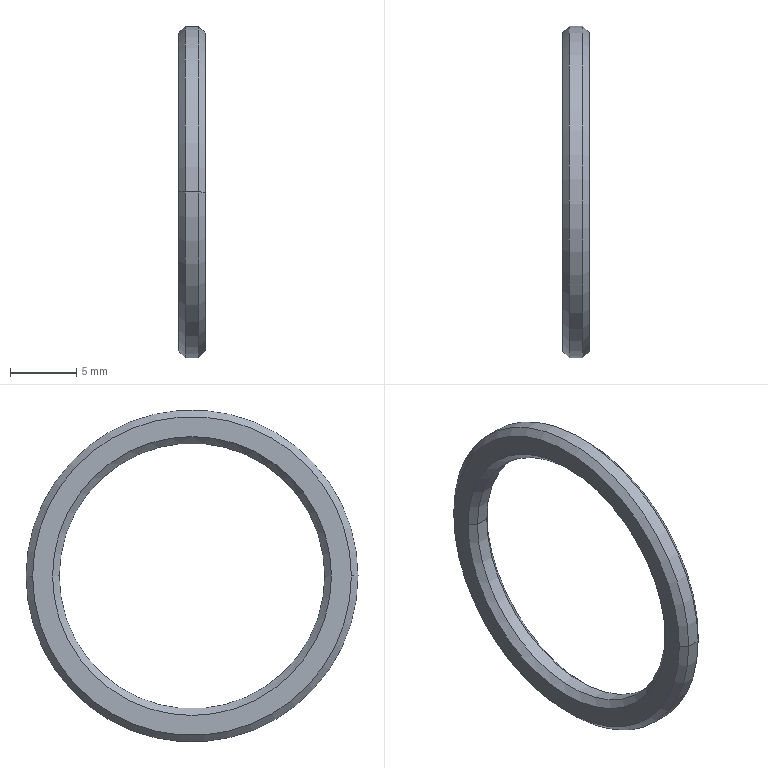Part | SolidWorks | features BaseBody 1 | 1 solid | 14 faces | box 2 x 25 x 25 mm | volume 318.086 mm3 | cone 8 | cylinder 4 | plane 2 | commonest cylinder face diameters 20 x2 25 x2
STEP:
#1=CARTESIAN_POINT('',(2.,12.,0.));
#2=VERTEX_POINT('',#1);
#3=CARTESIAN_POINT('',(2.,-12.,0.));
#4=VERTEX_POINT('',#3);
#5=CARTESIAN_POINT('',(2.,0.,0.));
#6=DIRECTION('',(1.,0.,0.));
#7=DIRECTION('',(0.,-1.,0.));
#8=AXIS2_PLACEMENT_3D('',#5,#6,#7);
#9=CIRCLE('',#8,12.);
#10=EDGE_CURVE('',#2,#4,#9,.T.);
#11=ORIENTED_EDGE('',*,*,#10,.F.);
#12=CARTESIAN_POINT('',(1.5,12.5,0.));
#13=VERTEX_POINT('',#12);
#14=CARTESIAN_POINT('',(1.5,12.5,0.));
#15=DIRECTION('',(-0.7071,0.7071,0.));
#16=VECTOR('',#15,1000.);
#17=LINE('',#14,#16);
#18=EDGE_CURVE('',#2,#13,#17,.T.);
#19=ORIENTED_EDGE('',*,*,#18,.T.);
#20=CARTESIAN_POINT('',(1.5,-12.5,0.));
#21=VERTEX_POINT('',#20);
#22=CARTESIAN_POINT('',(1.5,0.,0.));
#23=DIRECTION('',(1.,0.,0.));
#24=DIRECTION('',(0.,-1.,0.));
#25=AXIS2_PLACEMENT_3D('',#22,#23,#24);
#26=CIRCLE('',#25,12.5);
#27=EDGE_CURVE('',#13,#21,#26,.T.);
#28=ORIENTED_EDGE('',*,*,#27,.T.);
#29=CARTESIAN_POINT('',(1.5,-12.5,0.));
#30=DIRECTION('',(-0.7071,-0.7071,0.));
#31=VECTOR('',#30,1000.);
#32=LINE('',#29,#31);
#33=EDGE_CURVE('',#4,#21,#32,.T.);
#34=ORIENTED_EDGE('',*,*,#33,.F.);
#35=EDGE_LOOP('',(#11,#19,#28,#34));
#36=FACE_OUTER_BOUND('',#35,.T.);
#37=CARTESIAN_POINT('',(1.5,0.,0.));
#38=DIRECTION('',(-1.,0.,0.));
#39=DIRECTION('',(0.,-1.,0.));
#40=AXIS2_PLACEMENT_3D('',#37,#38,#39);
#41=CONICAL_SURFACE('',#40,12.5,0.7854);
#42=ADVANCED_FACE('',(#36),#41,.T.);
#43=CARTESIAN_POINT('',(1.5,-10.,0.));
#44=VERTEX_POINT('',#43);
#45=CARTESIAN_POINT('',(1.5,10.,0.));
#46=VERTEX_POINT('',#45);
#47=CARTESIAN_POINT('',(1.5,0.,0.));
#48=DIRECTION('',(1.,0.,0.));
#49=DIRECTION('',(0.,1.,0.));
#50=AXIS2_PLACEMENT_3D('',#47,#48,#49);
#51=CIRCLE('',#50,10.);
#52=EDGE_CURVE('',#44,#46,#51,.T.);
#53=ORIENTED_EDGE('',*,*,#52,.F.);
#54=CARTESIAN_POINT('',(2.,-10.5,0.));
#55=VERTEX_POINT('',#54);
#56=CARTESIAN_POINT('',(2.,-10.5,0.));
#57=DIRECTION('',(0.7071,-0.7071,0.));
#58=VECTOR('',#57,1000.);
#59=LINE('',#56,#58);
#60=EDGE_CURVE('',#44,#55,#59,.T.);
#61=ORIENTED_EDGE('',*,*,#60,.T.);
#62=CARTESIAN_POINT('',(2.,10.5,0.));
#63=VERTEX_POINT('',#62);
#64=CARTESIAN_POINT('',(2.,0.,0.));
#65=DIRECTION('',(-1.,0.,0.));
#66=DIRECTION('',(0.,1.,0.));
#67=AXIS2_PLACEMENT_3D('',#64,#65,#66);
#68=CIRCLE('',#67,10.5);
#69=EDGE_CURVE('',#63,#55,#68,.T.);
#70=ORIENTED_EDGE('',*,*,#69,.F.);
#71=CARTESIAN_POINT('',(2.,10.5,0.));
#72=DIRECTION('',(0.7071,0.7071,0.));
#73=VECTOR('',#72,1000.);
#74=LINE('',#71,#73);
#75=EDGE_CURVE('',#46,#63,#74,.T.);
#76=ORIENTED_EDGE('',*,*,#75,.F.);
#77=EDGE_LOOP('',(#53,#61,#70,#76));
#78=FACE_OUTER_BOUND('',#77,.T.);
#79=CARTESIAN_POINT('',(2.,0.,0.));
#80=DIRECTION('',(1.,0.,0.));
#81=DIRECTION('',(0.,1.,0.));
#82=AXIS2_PLACEMENT_3D('',#79,#80,#81);
#83=CONICAL_SURFACE('',#82,10.5,0.7854);
#84=ADVANCED_FACE('',(#78),#83,.F.);
#85=CARTESIAN_POINT('',(0.5,12.5,0.));
#86=VERTEX_POINT('',#85);
#87=CARTESIAN_POINT('',(0.5,-12.5,0.));
#88=VERTEX_POINT('',#87);
#89=CARTESIAN_POINT('',(0.5,0.,0.));
#90=DIRECTION('',(1.,0.,0.));
#91=DIRECTION('',(0.,1.,0.));
#92=AXIS2_PLACEMENT_3D('',#89,#90,#91);
#93=CIRCLE('',#92,12.5);
#94=EDGE_CURVE('',#86,#88,#93,.T.);
#95=ORIENTED_EDGE('',*,*,#94,.T.);
#96=CARTESIAN_POINT('',(-3.,-12.5,0.));
#97=DIRECTION('',(1.,0.,0.));
#98=VECTOR('',#97,1000.);
#99=LINE('',#96,#98);
#100=EDGE_CURVE('',#88,#21,#99,.T.);
#101=ORIENTED_EDGE('',*,*,#100,.T.);
#102=ORIENTED_EDGE('',*,*,#27,.F.);
#103=CARTESIAN_POINT('',(-3.,12.5,0.));
#104=DIRECTION('',(1.,0.,0.));
#105=VECTOR('',#104,1000.);
#106=LINE('',#103,#105);
#107=EDGE_CURVE('',#86,#13,#106,.T.);
#108=ORIENTED_EDGE('',*,*,#107,.F.);
#109=EDGE_LOOP('',(#95,#101,#102,#108));
#110=FACE_OUTER_BOUND('',#109,.T.);
#111=CARTESIAN_POINT('',(-3.,0.,0.));
#112=DIRECTION('',(1.,0.,0.));
#113=DIRECTION('',(0.,1.,0.));
#114=AXIS2_PLACEMENT_3D('',#111,#112,#113);
#115=CYLINDRICAL_SURFACE('',#114,12.5);
#116=ADVANCED_FACE('',(#110),#115,.T.);
#117=CARTESIAN_POINT('',(0.5,-10.,0.));
#118=VERTEX_POINT('',#117);
#119=CARTESIAN_POINT('',(0.5,10.,0.));
#120=VERTEX_POINT('',#119);
#121=CARTESIAN_POINT('',(0.5,0.,0.));
#122=DIRECTION('',(1.,0.,0.));
#123=DIRECTION('',(0.,1.,0.));
#124=AXIS2_PLACEMENT_3D('',#121,#122,#123);
#125=CIRCLE('',#124,10.);
#126=EDGE_CURVE('',#118,#120,#125,.T.);
#127=ORIENTED_EDGE('',*,*,#126,.F.);
#128=CARTESIAN_POINT('',(-3.,-10.,0.));
#129=DIRECTION('',(1.,0.,0.));
#130=VECTOR('',#129,1000.);
#131=LINE('',#128,#130);
#132=EDGE_CURVE('',#118,#44,#131,.T.);
#133=ORIENTED_EDGE('',*,*,#132,.T.);
#134=ORIENTED_EDGE('',*,*,#52,.T.);
#135=CARTESIAN_POINT('',(-3.,10.,0.));
#136=DIRECTION('',(1.,0.,0.));
#137=VECTOR('',#136,1000.);
#138=LINE('',#135,#137);
#139=EDGE_CURVE('',#120,#46,#138,.T.);
#140=ORIENTED_EDGE('',*,*,#139,.F.);
#141=EDGE_LOOP('',(#127,#133,#134,#140));
#142=FACE_OUTER_BOUND('',#141,.T.);
#143=CARTESIAN_POINT('',(-3.,0.,0.));
#144=DIRECTION('',(1.,0.,0.));
#145=DIRECTION('',(0.,1.,0.));
#146=AXIS2_PLACEMENT_3D('',#143,#144,#145);
#147=CYLINDRICAL_SURFACE('',#146,10.);
#148=ADVANCED_FACE('',(#142),#147,.F.);
#149=CARTESIAN_POINT('',(0.,12.,0.));
#150=VERTEX_POINT('',#149);
#151=CARTESIAN_POINT('',(0.,-12.,0.));
#152=VERTEX_POINT('',#151);
#153=CARTESIAN_POINT('',(0.,0.,0.));
#154=DIRECTION('',(1.,0.,0.));
#155=DIRECTION('',(0.,1.,0.));
#156=AXIS2_PLACEMENT_3D('',#153,#154,#155);
#157=CIRCLE('',#156,12.);
#158=EDGE_CURVE('',#150,#152,#157,.T.);
#159=ORIENTED_EDGE('',*,*,#158,.T.);
#160=CARTESIAN_POINT('',(0.5,-12.5,0.));
#161=DIRECTION('',(0.7071,-0.7071,0.));
#162=VECTOR('',#161,1000.);
#163=LINE('',#160,#162);
#164=EDGE_CURVE('',#152,#88,#163,.T.);
#165=ORIENTED_EDGE('',*,*,#164,.T.);
#166=ORIENTED_EDGE('',*,*,#94,.F.);
#167=CARTESIAN_POINT('',(0.5,12.5,0.));
#168=DIRECTION('',(0.7071,0.7071,0.));
#169=VECTOR('',#168,1000.);
#170=LINE('',#167,#169);
#171=EDGE_CURVE('',#150,#86,#170,.T.);
#172=ORIENTED_EDGE('',*,*,#171,.F.);
#173=EDGE_LOOP('',(#159,#165,#166,#172));
#174=FACE_OUTER_BOUND('',#173,.T.);
#175=CARTESIAN_POINT('',(0.5,0.,0.));
#176=DIRECTION('',(1.,0.,0.));
#177=DIRECTION('',(0.,1.,0.));
#178=AXIS2_PLACEMENT_3D('',#175,#176,#177);
#179=CONICAL_SURFACE('',#178,12.5,0.7854);
#180=ADVANCED_FACE('',(#174),#179,.T.);
#181=ORIENTED_EDGE('',*,*,#126,.T.);
#182=CARTESIAN_POINT('',(0.,10.5,0.));
#183=VERTEX_POINT('',#182);
#184=CARTESIAN_POINT('',(0.,10.5,0.));
#185=DIRECTION('',(-0.7071,0.7071,0.));
#186=VECTOR('',#185,1000.);
#187=LINE('',#184,#186);
#188=EDGE_CURVE('',#120,#183,#187,.T.);
#189=ORIENTED_EDGE('',*,*,#188,.T.);
#190=CARTESIAN_POINT('',(0.,-10.5,0.));
#191=VERTEX_POINT('',#190);
#192=CARTESIAN_POINT('',(0.,0.,0.));
#193=DIRECTION('',(1.,0.,0.));
#194=DIRECTION('',(0.,-1.,0.));
#195=AXIS2_PLACEMENT_3D('',#192,#193,#194);
#196=CIRCLE('',#195,10.5);
#197=EDGE_CURVE('',#191,#183,#196,.T.);
#198=ORIENTED_EDGE('',*,*,#197,.F.);
#199=CARTESIAN_POINT('',(0.,-10.5,0.));
#200=DIRECTION('',(-0.7071,-0.7071,0.));
#201=VECTOR('',#200,1000.);
#202=LINE('',#199,#201);
#203=EDGE_CURVE('',#118,#191,#202,.T.);
#204=ORIENTED_EDGE('',*,*,#203,.F.);
#205=EDGE_LOOP('',(#181,#189,#198,#204));
#206=FACE_OUTER_BOUND('',#205,.T.);
#207=CARTESIAN_POINT('',(0.,0.,0.));
#208=DIRECTION('',(-1.,0.,0.));
#209=DIRECTION('',(0.,-1.,0.));
#210=AXIS2_PLACEMENT_3D('',#207,#208,#209);
#211=CONICAL_SURFACE('',#210,10.5,0.7854);
#212=ADVANCED_FACE('',(#206),#211,.F.);
#213=ORIENTED_EDGE('',*,*,#197,.T.);
#214=CARTESIAN_POINT('',(0.,0.,0.));
#215=DIRECTION('',(1.,0.,0.));
#216=DIRECTION('',(0.,-1.,0.));
#217=AXIS2_PLACEMENT_3D('',#214,#215,#216);
#218=CIRCLE('',#217,10.5);
#219=EDGE_CURVE('',#183,#191,#218,.T.);
#220=ORIENTED_EDGE('',*,*,#219,.T.);
#221=EDGE_LOOP('',(#213,#220));
#222=FACE_BOUND('',#221,.T.);
#223=ORIENTED_EDGE('',*,*,#158,.F.);
#224=CARTESIAN_POINT('',(0.,0.,0.));
#225=DIRECTION('',(1.,0.,0.));
#226=DIRECTION('',(0.,1.,0.));
#227=AXIS2_PLACEMENT_3D('',#224,#225,#226);
#228=CIRCLE('',#227,12.);
#229=EDGE_CURVE('',#152,#150,#228,.T.);
#230=ORIENTED_EDGE('',*,*,#229,.F.);
#231=EDGE_LOOP('',(#223,#230));
#232=FACE_OUTER_BOUND('',#231,.T.);
#233=CARTESIAN_POINT('',(0.,-10.5,0.));
#234=DIRECTION('',(-1.,0.,0.));
#235=DIRECTION('',(0.,1.,0.));
#236=AXIS2_PLACEMENT_3D('',#233,#234,#235);
#237=PLANE('',#236);
#238=ADVANCED_FACE('',(#222,#232),#237,.T.);
#239=ORIENTED_EDGE('',*,*,#69,.T.);
#240=CARTESIAN_POINT('',(2.,0.,0.));
#241=DIRECTION('',(-1.,0.,0.));
#242=DIRECTION('',(0.,1.,0.));
#243=AXIS2_PLACEMENT_3D('',#240,#241,#242);
#244=CIRCLE('',#243,10.5);
#245=EDGE_CURVE('',#55,#63,#244,.T.);
#246=ORIENTED_EDGE('',*,*,#245,.T.);
#247=EDGE_LOOP('',(#239,#246));
#248=FACE_BOUND('',#247,.T.);
#249=CARTESIAN_POINT('',(2.,0.,0.));
#250=DIRECTION('',(1.,0.,0.));
#251=DIRECTION('',(0.,-1.,0.));
#252=AXIS2_PLACEMENT_3D('',#249,#250,#251);
#253=CIRCLE('',#252,12.);
#254=EDGE_CURVE('',#4,#2,#253,.T.);
#255=ORIENTED_EDGE('',*,*,#254,.T.);
#256=ORIENTED_EDGE('',*,*,#10,.T.);
#257=EDGE_LOOP('',(#255,#256));
#258=FACE_OUTER_BOUND('',#257,.T.);
#259=CARTESIAN_POINT('',(2.,-12.,0.));
#260=DIRECTION('',(1.,0.,0.));
#261=DIRECTION('',(0.,1.,0.));
#262=AXIS2_PLACEMENT_3D('',#259,#260,#261);
#263=PLANE('',#262);
#264=ADVANCED_FACE('',(#248,#258),#263,.T.);
#265=ORIENTED_EDGE('',*,*,#188,.F.);
#266=CARTESIAN_POINT('',(0.5,0.,0.));
#267=DIRECTION('',(1.,0.,0.));
#268=DIRECTION('',(0.,1.,0.));
#269=AXIS2_PLACEMENT_3D('',#266,#267,#268);
#270=CIRCLE('',#269,10.);
#271=EDGE_CURVE('',#120,#118,#270,.T.);
#272=ORIENTED_EDGE('',*,*,#271,.T.);
#273=ORIENTED_EDGE('',*,*,#203,.T.);
#274=ORIENTED_EDGE('',*,*,#219,.F.);
#275=EDGE_LOOP('',(#265,#272,#273,#274));
#276=FACE_OUTER_BOUND('',#275,.T.);
#277=CARTESIAN_POINT('',(0.,0.,0.));
#278=DIRECTION('',(-1.,0.,0.));
#279=DIRECTION('',(0.,-1.,0.));
#280=AXIS2_PLACEMENT_3D('',#277,#278,#279);
#281=CONICAL_SURFACE('',#280,10.5,0.7854);
#282=ADVANCED_FACE('',(#276),#281,.F.);
#283=ORIENTED_EDGE('',*,*,#164,.F.);
#284=ORIENTED_EDGE('',*,*,#229,.T.);
#285=ORIENTED_EDGE('',*,*,#171,.T.);
#286=CARTESIAN_POINT('',(0.5,0.,0.));
#287=DIRECTION('',(1.,0.,0.));
#288=DIRECTION('',(0.,1.,0.));
#289=AXIS2_PLACEMENT_3D('',#286,#287,#288);
#290=CIRCLE('',#289,12.5);
#291=EDGE_CURVE('',#88,#86,#290,.T.);
#292=ORIENTED_EDGE('',*,*,#291,.F.);
#293=EDGE_LOOP('',(#283,#284,#285,#292));
#294=FACE_OUTER_BOUND('',#293,.T.);
#295=CARTESIAN_POINT('',(0.5,0.,0.));
#296=DIRECTION('',(1.,0.,0.));
#297=DIRECTION('',(0.,1.,0.));
#298=AXIS2_PLACEMENT_3D('',#295,#296,#297);
#299=CONICAL_SURFACE('',#298,12.5,0.7854);
#300=ADVANCED_FACE('',(#294),#299,.T.);
#301=ORIENTED_EDGE('',*,*,#132,.F.);
#302=ORIENTED_EDGE('',*,*,#271,.F.);
#303=ORIENTED_EDGE('',*,*,#139,.T.);
#304=CARTESIAN_POINT('',(1.5,0.,0.));
#305=DIRECTION('',(1.,0.,0.));
#306=DIRECTION('',(0.,1.,0.));
#307=AXIS2_PLACEMENT_3D('',#304,#305,#306);
#308=CIRCLE('',#307,10.);
#309=EDGE_CURVE('',#46,#44,#308,.T.);
#310=ORIENTED_EDGE('',*,*,#309,.T.);
#311=EDGE_LOOP('',(#301,#302,#303,#310));
#312=FACE_OUTER_BOUND('',#311,.T.);
#313=CARTESIAN_POINT('',(-3.,0.,0.));
#314=DIRECTION('',(1.,0.,0.));
#315=DIRECTION('',(0.,1.,0.));
#316=AXIS2_PLACEMENT_3D('',#313,#314,#315);
#317=CYLINDRICAL_SURFACE('',#316,10.);
#318=ADVANCED_FACE('',(#312),#317,.F.);
#319=ORIENTED_EDGE('',*,*,#100,.F.);
#320=ORIENTED_EDGE('',*,*,#291,.T.);
#321=ORIENTED_EDGE('',*,*,#107,.T.);
#322=CARTESIAN_POINT('',(1.5,0.,0.));
#323=DIRECTION('',(1.,0.,0.));
#324=DIRECTION('',(0.,-1.,0.));
#325=AXIS2_PLACEMENT_3D('',#322,#323,#324);
#326=CIRCLE('',#325,12.5);
#327=EDGE_CURVE('',#21,#13,#326,.T.);
#328=ORIENTED_EDGE('',*,*,#327,.F.);
#329=EDGE_LOOP('',(#319,#320,#321,#328));
#330=FACE_OUTER_BOUND('',#329,.T.);
#331=CARTESIAN_POINT('',(-3.,0.,0.));
#332=DIRECTION('',(1.,0.,0.));
#333=DIRECTION('',(0.,1.,0.));
#334=AXIS2_PLACEMENT_3D('',#331,#332,#333);
#335=CYLINDRICAL_SURFACE('',#334,12.5);
#336=ADVANCED_FACE('',(#330),#335,.T.);
#337=ORIENTED_EDGE('',*,*,#60,.F.);
#338=ORIENTED_EDGE('',*,*,#309,.F.);
#339=ORIENTED_EDGE('',*,*,#75,.T.);
#340=ORIENTED_EDGE('',*,*,#245,.F.);
#341=EDGE_LOOP('',(#337,#338,#339,#340));
#342=FACE_OUTER_BOUND('',#341,.T.);
#343=CARTESIAN_POINT('',(2.,0.,0.));
#344=DIRECTION('',(1.,0.,0.));
#345=DIRECTION('',(0.,1.,0.));
#346=AXIS2_PLACEMENT_3D('',#343,#344,#345);
#347=CONICAL_SURFACE('',#346,10.5,0.7854);
#348=ADVANCED_FACE('',(#342),#347,.F.);
#349=ORIENTED_EDGE('',*,*,#18,.F.);
#350=ORIENTED_EDGE('',*,*,#254,.F.);
#351=ORIENTED_EDGE('',*,*,#33,.T.);
#352=ORIENTED_EDGE('',*,*,#327,.T.);
#353=EDGE_LOOP('',(#349,#350,#351,#352));
#354=FACE_OUTER_BOUND('',#353,.T.);
#355=CARTESIAN_POINT('',(1.5,0.,0.));
#356=DIRECTION('',(-1.,0.,0.));
#357=DIRECTION('',(0.,-1.,0.));
#358=AXIS2_PLACEMENT_3D('',#355,#356,#357);
#359=CONICAL_SURFACE('',#358,12.5,0.7854);
#360=ADVANCED_FACE('',(#354),#359,.T.);
#361=CLOSED_SHELL('',(#42,#84,#116,#148,#180,#212,#238,#264,#282,#300,#318,#336,#348,#360));
#362=MANIFOLD_SOLID_BREP('',#361);
#363=CARTESIAN_POINT('',(0.,0.,0.));
#364=DIRECTION('',(0.,0.,1.));
#365=DIRECTION('',(1.,0.,0.));
#366=AXIS2_PLACEMENT_3D('',#363,#364,#365);
#367=(LENGTH_UNIT()NAMED_UNIT(*)SI_UNIT(.MILLI.,.METRE.));
#368=UNCERTAINTY_MEASURE_WITH_UNIT(LENGTH_MEASURE(0.00001),#367,'','');
#369=(NAMED_UNIT(*)PLANE_ANGLE_UNIT()SI_UNIT($,.RADIAN.));
#370=(NAMED_UNIT(*)SI_UNIT($,.STERADIAN.)SOLID_ANGLE_UNIT());
#371=(GEOMETRIC_REPRESENTATION_CONTEXT(3)GLOBAL_UNCERTAINTY_ASSIGNED_CONTEXT((#368))GLOBAL_UNIT_ASSIGNED_CONTEXT((#367,#369,#370))REPRESENTATION_CONTEXT('',''));
#372=ADVANCED_BREP_SHAPE_REPRESENTATION('',(#362,#366),#371);